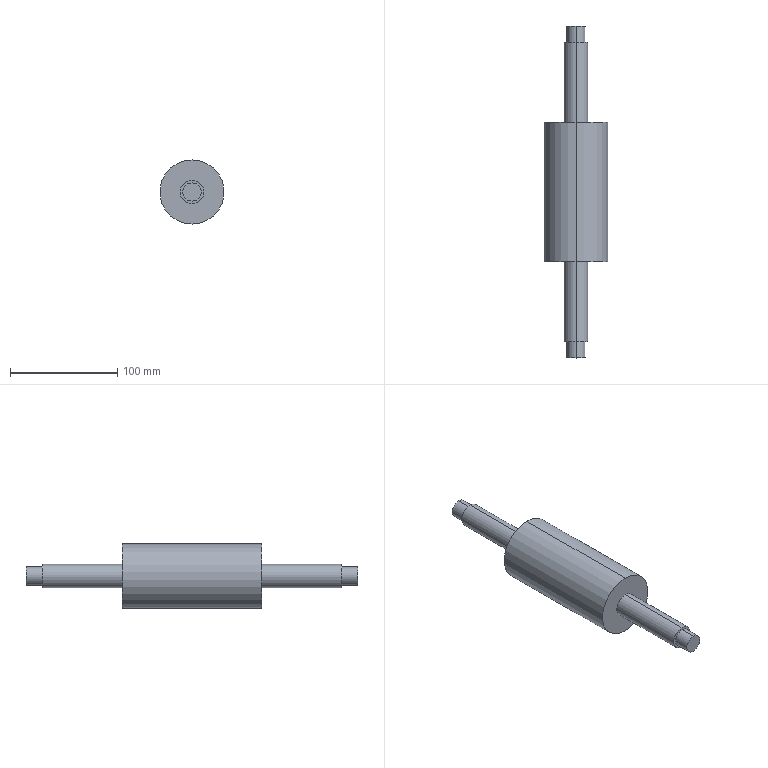Part | STEP file | A14-012 | 1 solid | 16 faces | box 60 x 310 x 60 mm | volume 431396 mm3 | cylinder 10 | plane 6 | commonest cylinder face diameters 17 x4 22 x4 60 x2
STEP:
#1=CARTESIAN_POINT('',(0.,0.,0.));
#2=DIRECTION('',(0.,0.,1.));
#3=DIRECTION('',(1.,0.,0.));
#4=AXIS2_PLACEMENT_3D('',#1,#2,#3);
#5=CARTESIAN_POINT('',(0.,15.,-8.5));
#6=VERTEX_POINT('',#5);
#7=CARTESIAN_POINT('',(0.,15.,8.5));
#8=VERTEX_POINT('',#7);
#9=CARTESIAN_POINT('',(0.,15.,0.));
#10=DIRECTION('',(0.,-1.,0.));
#11=DIRECTION('',(0.,0.,-1.));
#12=AXIS2_PLACEMENT_3D('',#9,#10,#11);
#13=CIRCLE('',#12,8.5);
#14=CARTESIAN_POINT('',(0.,0.,0.));
#15=DIRECTION('',(0.,-1.,0.));
#16=DIRECTION('',(0.,0.,-1.));
#17=AXIS2_PLACEMENT_3D('',#14,#15,#16);
#18=CYLINDRICAL_SURFACE('',#17,8.5);
#19=CARTESIAN_POINT('',(0.,-15.));
#20=DIRECTION('',(1.,0.));
#21=VECTOR('',#20,1.);
#22=LINE('',#19,#21);
#23=(GEOMETRIC_REPRESENTATION_CONTEXT(2)PARAMETRIC_REPRESENTATION_CONTEXT()REPRESENTATION_CONTEXT('',''));
#24=DEFINITIONAL_REPRESENTATION('',(#22),#23);
#25=PCURVE('',#18,#24);
#26=CARTESIAN_POINT('',(11.,15.,0.));
#27=DIRECTION('',(0.,-1.,0.));
#28=DIRECTION('',(0.,0.,-1.));
#29=AXIS2_PLACEMENT_3D('',#26,#27,#28);
#30=PLANE('',#29);
#31=CARTESIAN_POINT('',(0.,-11.));
#32=DIRECTION('',(1.,0.));
#33=AXIS2_PLACEMENT_2D('',#31,#32);
#34=CIRCLE('',#33,8.5);
#35=(GEOMETRIC_REPRESENTATION_CONTEXT(2)PARAMETRIC_REPRESENTATION_CONTEXT()REPRESENTATION_CONTEXT('',''));
#36=DEFINITIONAL_REPRESENTATION('',(#34),#35);
#37=PCURVE('',#30,#36);
#38=SURFACE_CURVE('',#13,(#25,#37),.PCURVE_S1.);
#39=EDGE_CURVE('',#6,#8,#38,.T.);
#40=ORIENTED_EDGE('',*,*,#39,.T.);
#41=CARTESIAN_POINT('',(0.,0.,8.5));
#42=VERTEX_POINT('',#41);
#43=CARTESIAN_POINT('',(0.,0.,8.5));
#44=DIRECTION('',(0.,-1.,0.));
#45=VECTOR('',#44,1.);
#46=LINE('',#43,#45);
#47=CARTESIAN_POINT('',(3.142,0.));
#48=DIRECTION('',(0.,1.));
#49=VECTOR('',#48,1.);
#50=LINE('',#47,#49);
#51=(GEOMETRIC_REPRESENTATION_CONTEXT(2)PARAMETRIC_REPRESENTATION_CONTEXT()REPRESENTATION_CONTEXT('',''));
#52=DEFINITIONAL_REPRESENTATION('',(#50),#51);
#53=PCURVE('',#18,#52);
#54=CARTESIAN_POINT('',(0.,0.,0.));
#55=DIRECTION('',(0.,-1.,0.));
#56=DIRECTION('',(0.,0.,-1.));
#57=AXIS2_PLACEMENT_3D('',#54,#55,#56);
#58=CYLINDRICAL_SURFACE('',#57,8.5);
#59=CARTESIAN_POINT('',(3.142,0.));
#60=DIRECTION('',(0.,1.));
#61=VECTOR('',#60,1.);
#62=LINE('',#59,#61);
#63=(GEOMETRIC_REPRESENTATION_CONTEXT(2)PARAMETRIC_REPRESENTATION_CONTEXT()REPRESENTATION_CONTEXT('',''));
#64=DEFINITIONAL_REPRESENTATION('',(#62),#63);
#65=PCURVE('',#58,#64);
#66=SURFACE_CURVE('',#46,(#53,#65),.PCURVE_S1.);
#67=EDGE_CURVE('',#8,#42,#66,.T.);
#68=ORIENTED_EDGE('',*,*,#67,.T.);
#69=CARTESIAN_POINT('',(0.,0.,-8.5));
#70=VERTEX_POINT('',#69);
#71=CARTESIAN_POINT('',(0.,0.,0.));
#72=DIRECTION('',(0.,-1.,0.));
#73=DIRECTION('',(0.,0.,-1.));
#74=AXIS2_PLACEMENT_3D('',#71,#72,#73);
#75=CIRCLE('',#74,8.5);
#76=CARTESIAN_POINT('',(0.,0.));
#77=DIRECTION('',(1.,0.));
#78=VECTOR('',#77,1.);
#79=LINE('',#76,#78);
#80=(GEOMETRIC_REPRESENTATION_CONTEXT(2)PARAMETRIC_REPRESENTATION_CONTEXT()REPRESENTATION_CONTEXT('',''));
#81=DEFINITIONAL_REPRESENTATION('',(#79),#80);
#82=PCURVE('',#18,#81);
#83=CARTESIAN_POINT('',(8.5,0.,0.));
#84=DIRECTION('',(0.,-1.,0.));
#85=DIRECTION('',(0.,0.,-1.));
#86=AXIS2_PLACEMENT_3D('',#83,#84,#85);
#87=PLANE('',#86);
#88=CARTESIAN_POINT('',(0.,-8.5));
#89=DIRECTION('',(1.,0.));
#90=AXIS2_PLACEMENT_2D('',#88,#89);
#91=CIRCLE('',#90,8.5);
#92=(GEOMETRIC_REPRESENTATION_CONTEXT(2)PARAMETRIC_REPRESENTATION_CONTEXT()REPRESENTATION_CONTEXT('',''));
#93=DEFINITIONAL_REPRESENTATION('',(#91),#92);
#94=PCURVE('',#87,#93);
#95=SURFACE_CURVE('',#75,(#82,#94),.PCURVE_S1.);
#96=EDGE_CURVE('',#70,#42,#95,.T.);
#97=ORIENTED_EDGE('',*,*,#96,.F.);
#98=CARTESIAN_POINT('',(0.,0.,-8.5));
#99=DIRECTION('',(0.,-1.,0.));
#100=VECTOR('',#99,1.);
#101=LINE('',#98,#100);
#102=CARTESIAN_POINT('',(0.,0.));
#103=DIRECTION('',(0.,1.));
#104=VECTOR('',#103,1.);
#105=LINE('',#102,#104);
#106=(GEOMETRIC_REPRESENTATION_CONTEXT(2)PARAMETRIC_REPRESENTATION_CONTEXT()REPRESENTATION_CONTEXT('',''));
#107=DEFINITIONAL_REPRESENTATION('',(#105),#106);
#108=PCURVE('',#18,#107);
#109=CARTESIAN_POINT('',(6.283,0.));
#110=DIRECTION('',(0.,1.));
#111=VECTOR('',#110,1.);
#112=LINE('',#109,#111);
#113=(GEOMETRIC_REPRESENTATION_CONTEXT(2)PARAMETRIC_REPRESENTATION_CONTEXT()REPRESENTATION_CONTEXT('',''));
#114=DEFINITIONAL_REPRESENTATION('',(#112),#113);
#115=PCURVE('',#58,#114);
#116=SURFACE_CURVE('',#101,(#108,#115),.PCURVE_S1.);
#117=EDGE_CURVE('',#6,#70,#116,.T.);
#118=ORIENTED_EDGE('',*,*,#117,.F.);
#119=EDGE_LOOP('',(#40,#68,#97,#118));
#120=FACE_BOUND('',#119,.T.);
#121=ADVANCED_FACE('',(#120),#18,.T.);
#122=CARTESIAN_POINT('',(0.,90.,-11.));
#123=VERTEX_POINT('',#122);
#124=CARTESIAN_POINT('',(0.,90.,11.));
#125=VERTEX_POINT('',#124);
#126=CARTESIAN_POINT('',(0.,90.,0.));
#127=DIRECTION('',(0.,-1.,0.));
#128=DIRECTION('',(0.,0.,-1.));
#129=AXIS2_PLACEMENT_3D('',#126,#127,#128);
#130=CIRCLE('',#129,11.);
#131=CARTESIAN_POINT('',(0.,0.,0.));
#132=DIRECTION('',(0.,-1.,0.));
#133=DIRECTION('',(0.,0.,-1.));
#134=AXIS2_PLACEMENT_3D('',#131,#132,#133);
#135=CYLINDRICAL_SURFACE('',#134,11.);
#136=CARTESIAN_POINT('',(0.,-90.));
#137=DIRECTION('',(1.,0.));
#138=VECTOR('',#137,1.);
#139=LINE('',#136,#138);
#140=(GEOMETRIC_REPRESENTATION_CONTEXT(2)PARAMETRIC_REPRESENTATION_CONTEXT()REPRESENTATION_CONTEXT('',''));
#141=DEFINITIONAL_REPRESENTATION('',(#139),#140);
#142=PCURVE('',#135,#141);
#143=CARTESIAN_POINT('',(30.,90.,0.));
#144=DIRECTION('',(0.,-1.,0.));
#145=DIRECTION('',(0.,0.,-1.));
#146=AXIS2_PLACEMENT_3D('',#143,#144,#145);
#147=PLANE('',#146);
#148=CARTESIAN_POINT('',(0.,-30.));
#149=DIRECTION('',(1.,0.));
#150=AXIS2_PLACEMENT_2D('',#148,#149);
#151=CIRCLE('',#150,11.);
#152=(GEOMETRIC_REPRESENTATION_CONTEXT(2)PARAMETRIC_REPRESENTATION_CONTEXT()REPRESENTATION_CONTEXT('',''));
#153=DEFINITIONAL_REPRESENTATION('',(#151),#152);
#154=PCURVE('',#147,#153);
#155=SURFACE_CURVE('',#130,(#142,#154),.PCURVE_S1.);
#156=EDGE_CURVE('',#123,#125,#155,.T.);
#157=ORIENTED_EDGE('',*,*,#156,.T.);
#158=CARTESIAN_POINT('',(0.,15.,11.));
#159=VERTEX_POINT('',#158);
#160=CARTESIAN_POINT('',(0.,0.,11.));
#161=DIRECTION('',(0.,-1.,0.));
#162=VECTOR('',#161,1.);
#163=LINE('',#160,#162);
#164=CARTESIAN_POINT('',(3.142,0.));
#165=DIRECTION('',(0.,1.));
#166=VECTOR('',#165,1.);
#167=LINE('',#164,#166);
#168=(GEOMETRIC_REPRESENTATION_CONTEXT(2)PARAMETRIC_REPRESENTATION_CONTEXT()REPRESENTATION_CONTEXT('',''));
#169=DEFINITIONAL_REPRESENTATION('',(#167),#168);
#170=PCURVE('',#135,#169);
#171=CARTESIAN_POINT('',(0.,0.,0.));
#172=DIRECTION('',(0.,-1.,0.));
#173=DIRECTION('',(0.,0.,-1.));
#174=AXIS2_PLACEMENT_3D('',#171,#172,#173);
#175=CYLINDRICAL_SURFACE('',#174,11.);
#176=CARTESIAN_POINT('',(3.142,0.));
#177=DIRECTION('',(0.,1.));
#178=VECTOR('',#177,1.);
#179=LINE('',#176,#178);
#180=(GEOMETRIC_REPRESENTATION_CONTEXT(2)PARAMETRIC_REPRESENTATION_CONTEXT()REPRESENTATION_CONTEXT('',''));
#181=DEFINITIONAL_REPRESENTATION('',(#179),#180);
#182=PCURVE('',#175,#181);
#183=SURFACE_CURVE('',#163,(#170,#182),.PCURVE_S1.);
#184=EDGE_CURVE('',#125,#159,#183,.T.);
#185=ORIENTED_EDGE('',*,*,#184,.T.);
#186=CARTESIAN_POINT('',(0.,15.,-11.));
#187=VERTEX_POINT('',#186);
#188=CARTESIAN_POINT('',(0.,15.,0.));
#189=DIRECTION('',(0.,-1.,0.));
#190=DIRECTION('',(0.,0.,-1.));
#191=AXIS2_PLACEMENT_3D('',#188,#189,#190);
#192=CIRCLE('',#191,11.);
#193=CARTESIAN_POINT('',(0.,-15.));
#194=DIRECTION('',(1.,0.));
#195=VECTOR('',#194,1.);
#196=LINE('',#193,#195);
#197=(GEOMETRIC_REPRESENTATION_CONTEXT(2)PARAMETRIC_REPRESENTATION_CONTEXT()REPRESENTATION_CONTEXT('',''));
#198=DEFINITIONAL_REPRESENTATION('',(#196),#197);
#199=PCURVE('',#135,#198);
#200=CARTESIAN_POINT('',(0.,-11.));
#201=DIRECTION('',(1.,0.));
#202=AXIS2_PLACEMENT_2D('',#200,#201);
#203=CIRCLE('',#202,11.);
#204=(GEOMETRIC_REPRESENTATION_CONTEXT(2)PARAMETRIC_REPRESENTATION_CONTEXT()REPRESENTATION_CONTEXT('',''));
#205=DEFINITIONAL_REPRESENTATION('',(#203),#204);
#206=PCURVE('',#30,#205);
#207=SURFACE_CURVE('',#192,(#199,#206),.PCURVE_S1.);
#208=EDGE_CURVE('',#187,#159,#207,.T.);
#209=ORIENTED_EDGE('',*,*,#208,.F.);
#210=CARTESIAN_POINT('',(0.,0.,-11.));
#211=DIRECTION('',(0.,-1.,0.));
#212=VECTOR('',#211,1.);
#213=LINE('',#210,#212);
#214=CARTESIAN_POINT('',(0.,0.));
#215=DIRECTION('',(0.,1.));
#216=VECTOR('',#215,1.);
#217=LINE('',#214,#216);
#218=(GEOMETRIC_REPRESENTATION_CONTEXT(2)PARAMETRIC_REPRESENTATION_CONTEXT()REPRESENTATION_CONTEXT('',''));
#219=DEFINITIONAL_REPRESENTATION('',(#217),#218);
#220=PCURVE('',#135,#219);
#221=CARTESIAN_POINT('',(6.283,0.));
#222=DIRECTION('',(0.,1.));
#223=VECTOR('',#222,1.);
#224=LINE('',#221,#223);
#225=(GEOMETRIC_REPRESENTATION_CONTEXT(2)PARAMETRIC_REPRESENTATION_CONTEXT()REPRESENTATION_CONTEXT('',''));
#226=DEFINITIONAL_REPRESENTATION('',(#224),#225);
#227=PCURVE('',#175,#226);
#228=SURFACE_CURVE('',#213,(#220,#227),.PCURVE_S1.);
#229=EDGE_CURVE('',#123,#187,#228,.T.);
#230=ORIENTED_EDGE('',*,*,#229,.F.);
#231=EDGE_LOOP('',(#157,#185,#209,#230));
#232=FACE_BOUND('',#231,.T.);
#233=ADVANCED_FACE('',(#232),#135,.T.);
#234=CARTESIAN_POINT('',(0.,220.,-30.));
#235=VERTEX_POINT('',#234);
#236=CARTESIAN_POINT('',(0.,220.,30.));
#237=VERTEX_POINT('',#236);
#238=CARTESIAN_POINT('',(0.,220.,0.));
#239=DIRECTION('',(0.,-1.,0.));
#240=DIRECTION('',(0.,0.,-1.));
#241=AXIS2_PLACEMENT_3D('',#238,#239,#240);
#242=CIRCLE('',#241,30.);
#243=CARTESIAN_POINT('',(0.,0.,0.));
#244=DIRECTION('',(0.,-1.,0.));
#245=DIRECTION('',(0.,0.,-1.));
#246=AXIS2_PLACEMENT_3D('',#243,#244,#245);
#247=CYLINDRICAL_SURFACE('',#246,30.);
#248=CARTESIAN_POINT('',(0.,-220.));
#249=DIRECTION('',(1.,0.));
#250=VECTOR('',#249,1.);
#251=LINE('',#248,#250);
#252=(GEOMETRIC_REPRESENTATION_CONTEXT(2)PARAMETRIC_REPRESENTATION_CONTEXT()REPRESENTATION_CONTEXT('',''));
#253=DEFINITIONAL_REPRESENTATION('',(#251),#252);
#254=PCURVE('',#247,#253);
#255=CARTESIAN_POINT('',(11.,220.,0.));
#256=DIRECTION('',(0.,1.,0.));
#257=DIRECTION('',(0.,0.,1.));
#258=AXIS2_PLACEMENT_3D('',#255,#256,#257);
#259=PLANE('',#258);
#260=CARTESIAN_POINT('',(-30.,-11.));
#261=CARTESIAN_POINT('',(-30.,40.962));
#262=CARTESIAN_POINT('',(15.,14.981));
#263=CARTESIAN_POINT('',(60.,-11.));
#264=CARTESIAN_POINT('',(15.,-36.981));
#265=CARTESIAN_POINT('',(-30.,-62.962));
#266=CARTESIAN_POINT('',(-30.,-11.));
#267=(BOUNDED_CURVE()B_SPLINE_CURVE(2,(#260,#261,#262,#263,#264,#265,#266),.UNSPECIFIED.,.T.,.F.)B_SPLINE_CURVE_WITH_KNOTS((1,2,2,2,2,1),(-2.094,0.,2.094,4.189,6.283,8.378),.UNSPECIFIED.)CURVE()GEOMETRIC_REPRESENTATION_ITEM()RATIONAL_B_SPLINE_CURVE((1.,0.5,1.,0.5,1.,0.5,1.))REPRESENTATION_ITEM(''));
#268=(GEOMETRIC_REPRESENTATION_CONTEXT(2)PARAMETRIC_REPRESENTATION_CONTEXT()REPRESENTATION_CONTEXT('',''));
#269=DEFINITIONAL_REPRESENTATION('',(#267),#268);
#270=PCURVE('',#259,#269);
#271=SURFACE_CURVE('',#242,(#254,#270),.PCURVE_S1.);
#272=EDGE_CURVE('',#235,#237,#271,.T.);
#273=ORIENTED_EDGE('',*,*,#272,.T.);
#274=CARTESIAN_POINT('',(0.,90.,30.));
#275=VERTEX_POINT('',#274);
#276=CARTESIAN_POINT('',(0.,0.,30.));
#277=DIRECTION('',(0.,-1.,0.));
#278=VECTOR('',#277,1.);
#279=LINE('',#276,#278);
#280=CARTESIAN_POINT('',(3.142,0.));
#281=DIRECTION('',(0.,1.));
#282=VECTOR('',#281,1.);
#283=LINE('',#280,#282);
#284=(GEOMETRIC_REPRESENTATION_CONTEXT(2)PARAMETRIC_REPRESENTATION_CONTEXT()REPRESENTATION_CONTEXT('',''));
#285=DEFINITIONAL_REPRESENTATION('',(#283),#284);
#286=PCURVE('',#247,#285);
#287=CARTESIAN_POINT('',(0.,0.,0.));
#288=DIRECTION('',(0.,-1.,0.));
#289=DIRECTION('',(0.,0.,-1.));
#290=AXIS2_PLACEMENT_3D('',#287,#288,#289);
#291=CYLINDRICAL_SURFACE('',#290,30.);
#292=CARTESIAN_POINT('',(3.142,0.));
#293=DIRECTION('',(0.,1.));
#294=VECTOR('',#293,1.);
#295=LINE('',#292,#294);
#296=(GEOMETRIC_REPRESENTATION_CONTEXT(2)PARAMETRIC_REPRESENTATION_CONTEXT()REPRESENTATION_CONTEXT('',''));
#297=DEFINITIONAL_REPRESENTATION('',(#295),#296);
#298=PCURVE('',#291,#297);
#299=SURFACE_CURVE('',#279,(#286,#298),.PCURVE_S1.);
#300=EDGE_CURVE('',#237,#275,#299,.T.);
#301=ORIENTED_EDGE('',*,*,#300,.T.);
#302=CARTESIAN_POINT('',(0.,90.,-30.));
#303=VERTEX_POINT('',#302);
#304=CARTESIAN_POINT('',(0.,90.,0.));
#305=DIRECTION('',(0.,-1.,0.));
#306=DIRECTION('',(0.,0.,-1.));
#307=AXIS2_PLACEMENT_3D('',#304,#305,#306);
#308=CIRCLE('',#307,30.);
#309=CARTESIAN_POINT('',(0.,-90.));
#310=DIRECTION('',(1.,0.));
#311=VECTOR('',#310,1.);
#312=LINE('',#309,#311);
#313=(GEOMETRIC_REPRESENTATION_CONTEXT(2)PARAMETRIC_REPRESENTATION_CONTEXT()REPRESENTATION_CONTEXT('',''));
#314=DEFINITIONAL_REPRESENTATION('',(#312),#313);
#315=PCURVE('',#247,#314);
#316=CARTESIAN_POINT('',(0.,-30.));
#317=DIRECTION('',(1.,0.));
#318=AXIS2_PLACEMENT_2D('',#316,#317);
#319=CIRCLE('',#318,30.);
#320=(GEOMETRIC_REPRESENTATION_CONTEXT(2)PARAMETRIC_REPRESENTATION_CONTEXT()REPRESENTATION_CONTEXT('',''));
#321=DEFINITIONAL_REPRESENTATION('',(#319),#320);
#322=PCURVE('',#147,#321);
#323=SURFACE_CURVE('',#308,(#315,#322),.PCURVE_S1.);
#324=EDGE_CURVE('',#303,#275,#323,.T.);
#325=ORIENTED_EDGE('',*,*,#324,.F.);
#326=CARTESIAN_POINT('',(0.,0.,-30.));
#327=DIRECTION('',(0.,-1.,0.));
#328=VECTOR('',#327,1.);
#329=LINE('',#326,#328);
#330=CARTESIAN_POINT('',(0.,0.));
#331=DIRECTION('',(0.,1.));
#332=VECTOR('',#331,1.);
#333=LINE('',#330,#332);
#334=(GEOMETRIC_REPRESENTATION_CONTEXT(2)PARAMETRIC_REPRESENTATION_CONTEXT()REPRESENTATION_CONTEXT('',''));
#335=DEFINITIONAL_REPRESENTATION('',(#333),#334);
#336=PCURVE('',#247,#335);
#337=CARTESIAN_POINT('',(6.283,0.));
#338=DIRECTION('',(0.,1.));
#339=VECTOR('',#338,1.);
#340=LINE('',#337,#339);
#341=(GEOMETRIC_REPRESENTATION_CONTEXT(2)PARAMETRIC_REPRESENTATION_CONTEXT()REPRESENTATION_CONTEXT('',''));
#342=DEFINITIONAL_REPRESENTATION('',(#340),#341);
#343=PCURVE('',#291,#342);
#344=SURFACE_CURVE('',#329,(#336,#343),.PCURVE_S1.);
#345=EDGE_CURVE('',#235,#303,#344,.T.);
#346=ORIENTED_EDGE('',*,*,#345,.F.);
#347=EDGE_LOOP('',(#273,#301,#325,#346));
#348=FACE_BOUND('',#347,.T.);
#349=ADVANCED_FACE('',(#348),#247,.T.);
#350=CARTESIAN_POINT('',(0.,295.,-11.));
#351=VERTEX_POINT('',#350);
#352=CARTESIAN_POINT('',(0.,295.,11.));
#353=VERTEX_POINT('',#352);
#354=CARTESIAN_POINT('',(0.,295.,0.));
#355=DIRECTION('',(0.,-1.,0.));
#356=DIRECTION('',(0.,0.,-1.));
#357=AXIS2_PLACEMENT_3D('',#354,#355,#356);
#358=CIRCLE('',#357,11.);
#359=CARTESIAN_POINT('',(0.,0.,0.));
#360=DIRECTION('',(0.,-1.,0.));
#361=DIRECTION('',(0.,0.,-1.));
#362=AXIS2_PLACEMENT_3D('',#359,#360,#361);
#363=CYLINDRICAL_SURFACE('',#362,11.);
#364=CARTESIAN_POINT('',(0.,-295.));
#365=DIRECTION('',(1.,0.));
#366=VECTOR('',#365,1.);
#367=LINE('',#364,#366);
#368=(GEOMETRIC_REPRESENTATION_CONTEXT(2)PARAMETRIC_REPRESENTATION_CONTEXT()REPRESENTATION_CONTEXT('',''));
#369=DEFINITIONAL_REPRESENTATION('',(#367),#368);
#370=PCURVE('',#363,#369);
#371=CARTESIAN_POINT('',(8.5,295.,0.));
#372=DIRECTION('',(0.,1.,0.));
#373=DIRECTION('',(0.,0.,1.));
#374=AXIS2_PLACEMENT_3D('',#371,#372,#373);
#375=PLANE('',#374);
#376=CARTESIAN_POINT('',(-11.,-8.5));
#377=CARTESIAN_POINT('',(-11.,10.553));
#378=CARTESIAN_POINT('',(5.5,1.026));
#379=CARTESIAN_POINT('',(22.,-8.5));
#380=CARTESIAN_POINT('',(5.5,-18.026));
#381=CARTESIAN_POINT('',(-11.,-27.553));
#382=CARTESIAN_POINT('',(-11.,-8.5));
#383=(BOUNDED_CURVE()B_SPLINE_CURVE(2,(#376,#377,#378,#379,#380,#381,#382),.UNSPECIFIED.,.T.,.F.)B_SPLINE_CURVE_WITH_KNOTS((1,2,2,2,2,1),(-2.094,0.,2.094,4.189,6.283,8.378),.UNSPECIFIED.)CURVE()GEOMETRIC_REPRESENTATION_ITEM()RATIONAL_B_SPLINE_CURVE((1.,0.5,1.,0.5,1.,0.5,1.))REPRESENTATION_ITEM(''));
#384=(GEOMETRIC_REPRESENTATION_CONTEXT(2)PARAMETRIC_REPRESENTATION_CONTEXT()REPRESENTATION_CONTEXT('',''));
#385=DEFINITIONAL_REPRESENTATION('',(#383),#384);
#386=PCURVE('',#375,#385);
#387=SURFACE_CURVE('',#358,(#370,#386),.PCURVE_S1.);
#388=EDGE_CURVE('',#351,#353,#387,.T.);
#389=ORIENTED_EDGE('',*,*,#388,.T.);
#390=CARTESIAN_POINT('',(0.,220.,11.));
#391=VERTEX_POINT('',#390);
#392=CARTESIAN_POINT('',(0.,0.,11.));
#393=DIRECTION('',(0.,-1.,0.));
#394=VECTOR('',#393,1.);
#395=LINE('',#392,#394);
#396=CARTESIAN_POINT('',(3.142,0.));
#397=DIRECTION('',(0.,1.));
#398=VECTOR('',#397,1.);
#399=LINE('',#396,#398);
#400=(GEOMETRIC_REPRESENTATION_CONTEXT(2)PARAMETRIC_REPRESENTATION_CONTEXT()REPRESENTATION_CONTEXT('',''));
#401=DEFINITIONAL_REPRESENTATION('',(#399),#400);
#402=PCURVE('',#363,#401);
#403=CARTESIAN_POINT('',(0.,0.,0.));
#404=DIRECTION('',(0.,-1.,0.));
#405=DIRECTION('',(0.,0.,-1.));
#406=AXIS2_PLACEMENT_3D('',#403,#404,#405);
#407=CYLINDRICAL_SURFACE('',#406,11.);
#408=CARTESIAN_POINT('',(3.142,0.));
#409=DIRECTION('',(0.,1.));
#410=VECTOR('',#409,1.);
#411=LINE('',#408,#410);
#412=(GEOMETRIC_REPRESENTATION_CONTEXT(2)PARAMETRIC_REPRESENTATION_CONTEXT()REPRESENTATION_CONTEXT('',''));
#413=DEFINITIONAL_REPRESENTATION('',(#411),#412);
#414=PCURVE('',#407,#413);
#415=SURFACE_CURVE('',#395,(#402,#414),.PCURVE_S1.);
#416=EDGE_CURVE('',#353,#391,#415,.T.);
#417=ORIENTED_EDGE('',*,*,#416,.T.);
#418=CARTESIAN_POINT('',(0.,220.,-11.));
#419=VERTEX_POINT('',#418);
#420=CARTESIAN_POINT('',(0.,220.,0.));
#421=DIRECTION('',(0.,-1.,0.));
#422=DIRECTION('',(0.,0.,-1.));
#423=AXIS2_PLACEMENT_3D('',#420,#421,#422);
#424=CIRCLE('',#423,11.);
#425=CARTESIAN_POINT('',(0.,-220.));
#426=DIRECTION('',(1.,0.));
#427=VECTOR('',#426,1.);
#428=LINE('',#425,#427);
#429=(GEOMETRIC_REPRESENTATION_CONTEXT(2)PARAMETRIC_REPRESENTATION_CONTEXT()REPRESENTATION_CONTEXT('',''));
#430=DEFINITIONAL_REPRESENTATION('',(#428),#429);
#431=PCURVE('',#363,#430);
#432=CARTESIAN_POINT('',(-11.,-11.));
#433=CARTESIAN_POINT('',(-11.,8.053));
#434=CARTESIAN_POINT('',(5.5,-1.474));
#435=CARTESIAN_POINT('',(22.,-11.));
#436=CARTESIAN_POINT('',(5.5,-20.526));
#437=CARTESIAN_POINT('',(-11.,-30.053));
#438=CARTESIAN_POINT('',(-11.,-11.));
#439=(BOUNDED_CURVE()B_SPLINE_CURVE(2,(#432,#433,#434,#435,#436,#437,#438),.UNSPECIFIED.,.T.,.F.)B_SPLINE_CURVE_WITH_KNOTS((1,2,2,2,2,1),(-2.094,0.,2.094,4.189,6.283,8.378),.UNSPECIFIED.)CURVE()GEOMETRIC_REPRESENTATION_ITEM()RATIONAL_B_SPLINE_CURVE((1.,0.5,1.,0.5,1.,0.5,1.))REPRESENTATION_ITEM(''));
#440=(GEOMETRIC_REPRESENTATION_CONTEXT(2)PARAMETRIC_REPRESENTATION_CONTEXT()REPRESENTATION_CONTEXT('',''));
#441=DEFINITIONAL_REPRESENTATION('',(#439),#440);
#442=PCURVE('',#259,#441);
#443=SURFACE_CURVE('',#424,(#431,#442),.PCURVE_S1.);
#444=EDGE_CURVE('',#419,#391,#443,.T.);
#445=ORIENTED_EDGE('',*,*,#444,.F.);
#446=CARTESIAN_POINT('',(0.,0.,-11.));
#447=DIRECTION('',(0.,-1.,0.));
#448=VECTOR('',#447,1.);
#449=LINE('',#446,#448);
#450=CARTESIAN_POINT('',(0.,0.));
#451=DIRECTION('',(0.,1.));
#452=VECTOR('',#451,1.);
#453=LINE('',#450,#452);
#454=(GEOMETRIC_REPRESENTATION_CONTEXT(2)PARAMETRIC_REPRESENTATION_CONTEXT()REPRESENTATION_CONTEXT('',''));
#455=DEFINITIONAL_REPRESENTATION('',(#453),#454);
#456=PCURVE('',#363,#455);
#457=CARTESIAN_POINT('',(6.283,0.));
#458=DIRECTION('',(0.,1.));
#459=VECTOR('',#458,1.);
#460=LINE('',#457,#459);
#461=(GEOMETRIC_REPRESENTATION_CONTEXT(2)PARAMETRIC_REPRESENTATION_CONTEXT()REPRESENTATION_CONTEXT('',''));
#462=DEFINITIONAL_REPRESENTATION('',(#460),#461);
#463=PCURVE('',#407,#462);
#464=SURFACE_CURVE('',#449,(#456,#463),.PCURVE_S1.);
#465=EDGE_CURVE('',#351,#419,#464,.T.);
#466=ORIENTED_EDGE('',*,*,#465,.F.);
#467=EDGE_LOOP('',(#389,#417,#445,#466));
#468=FACE_BOUND('',#467,.T.);
#469=ADVANCED_FACE('',(#468),#363,.T.);
#470=CARTESIAN_POINT('',(0.,310.,-8.5));
#471=VERTEX_POINT('',#470);
#472=CARTESIAN_POINT('',(0.,310.,8.5));
#473=VERTEX_POINT('',#472);
#474=CARTESIAN_POINT('',(0.,310.,0.));
#475=DIRECTION('',(0.,-1.,0.));
#476=DIRECTION('',(0.,0.,-1.));
#477=AXIS2_PLACEMENT_3D('',#474,#475,#476);
#478=CIRCLE('',#477,8.5);
#479=CARTESIAN_POINT('',(0.,0.,0.));
#480=DIRECTION('',(0.,-1.,0.));
#481=DIRECTION('',(0.,0.,-1.));
#482=AXIS2_PLACEMENT_3D('',#479,#480,#481);
#483=CYLINDRICAL_SURFACE('',#482,8.5);
#484=CARTESIAN_POINT('',(0.,-310.));
#485=DIRECTION('',(1.,0.));
#486=VECTOR('',#485,1.);
#487=LINE('',#484,#486);
#488=(GEOMETRIC_REPRESENTATION_CONTEXT(2)PARAMETRIC_REPRESENTATION_CONTEXT()REPRESENTATION_CONTEXT('',''));
#489=DEFINITIONAL_REPRESENTATION('',(#487),#488);
#490=PCURVE('',#483,#489);
#491=CARTESIAN_POINT('',(0.,310.,0.));
#492=DIRECTION('',(0.,1.,0.));
#493=DIRECTION('',(0.,0.,1.));
#494=AXIS2_PLACEMENT_3D('',#491,#492,#493);
#495=PLANE('',#494);
#496=CARTESIAN_POINT('',(-8.5,0.));
#497=CARTESIAN_POINT('',(-8.5,14.722));
#498=CARTESIAN_POINT('',(4.25,7.361));
#499=CARTESIAN_POINT('',(17.,0.));
#500=CARTESIAN_POINT('',(4.25,-7.361));
#501=CARTESIAN_POINT('',(-8.5,-14.722));
#502=CARTESIAN_POINT('',(-8.5,0.));
#503=(BOUNDED_CURVE()B_SPLINE_CURVE(2,(#496,#497,#498,#499,#500,#501,#502),.UNSPECIFIED.,.T.,.F.)B_SPLINE_CURVE_WITH_KNOTS((1,2,2,2,2,1),(-2.094,0.,2.094,4.189,6.283,8.378),.UNSPECIFIED.)CURVE()GEOMETRIC_REPRESENTATION_ITEM()RATIONAL_B_SPLINE_CURVE((1.,0.5,1.,0.5,1.,0.5,1.))REPRESENTATION_ITEM(''));
#504=(GEOMETRIC_REPRESENTATION_CONTEXT(2)PARAMETRIC_REPRESENTATION_CONTEXT()REPRESENTATION_CONTEXT('',''));
#505=DEFINITIONAL_REPRESENTATION('',(#503),#504);
#506=PCURVE('',#495,#505);
#507=SURFACE_CURVE('',#478,(#490,#506),.PCURVE_S1.);
#508=EDGE_CURVE('',#471,#473,#507,.T.);
#509=ORIENTED_EDGE('',*,*,#508,.T.);
#510=CARTESIAN_POINT('',(0.,295.,8.5));
#511=VERTEX_POINT('',#510);
#512=CARTESIAN_POINT('',(0.,0.,8.5));
#513=DIRECTION('',(0.,-1.,0.));
#514=VECTOR('',#513,1.);
#515=LINE('',#512,#514);
#516=CARTESIAN_POINT('',(3.142,0.));
#517=DIRECTION('',(0.,1.));
#518=VECTOR('',#517,1.);
#519=LINE('',#516,#518);
#520=(GEOMETRIC_REPRESENTATION_CONTEXT(2)PARAMETRIC_REPRESENTATION_CONTEXT()REPRESENTATION_CONTEXT('',''));
#521=DEFINITIONAL_REPRESENTATION('',(#519),#520);
#522=PCURVE('',#483,#521);
#523=CARTESIAN_POINT('',(0.,0.,0.));
#524=DIRECTION('',(0.,-1.,0.));
#525=DIRECTION('',(0.,0.,-1.));
#526=AXIS2_PLACEMENT_3D('',#523,#524,#525);
#527=CYLINDRICAL_SURFACE('',#526,8.5);
#528=CARTESIAN_POINT('',(3.142,0.));
#529=DIRECTION('',(0.,1.));
#530=VECTOR('',#529,1.);
#531=LINE('',#528,#530);
#532=(GEOMETRIC_REPRESENTATION_CONTEXT(2)PARAMETRIC_REPRESENTATION_CONTEXT()REPRESENTATION_CONTEXT('',''));
#533=DEFINITIONAL_REPRESENTATION('',(#531),#532);
#534=PCURVE('',#527,#533);
#535=SURFACE_CURVE('',#515,(#522,#534),.PCURVE_S1.);
#536=EDGE_CURVE('',#473,#511,#535,.T.);
#537=ORIENTED_EDGE('',*,*,#536,.T.);
#538=CARTESIAN_POINT('',(0.,295.,-8.5));
#539=VERTEX_POINT('',#538);
#540=CARTESIAN_POINT('',(0.,295.,0.));
#541=DIRECTION('',(0.,-1.,0.));
#542=DIRECTION('',(0.,0.,-1.));
#543=AXIS2_PLACEMENT_3D('',#540,#541,#542);
#544=CIRCLE('',#543,8.5);
#545=CARTESIAN_POINT('',(0.,-295.));
#546=DIRECTION('',(1.,0.));
#547=VECTOR('',#546,1.);
#548=LINE('',#545,#547);
#549=(GEOMETRIC_REPRESENTATION_CONTEXT(2)PARAMETRIC_REPRESENTATION_CONTEXT()REPRESENTATION_CONTEXT('',''));
#550=DEFINITIONAL_REPRESENTATION('',(#548),#549);
#551=PCURVE('',#483,#550);
#552=CARTESIAN_POINT('',(-8.5,-8.5));
#553=CARTESIAN_POINT('',(-8.5,6.222));
#554=CARTESIAN_POINT('',(4.25,-1.139));
#555=CARTESIAN_POINT('',(17.,-8.5));
#556=CARTESIAN_POINT('',(4.25,-15.861));
#557=CARTESIAN_POINT('',(-8.5,-23.222));
#558=CARTESIAN_POINT('',(-8.5,-8.5));
#559=(BOUNDED_CURVE()B_SPLINE_CURVE(2,(#552,#553,#554,#555,#556,#557,#558),.UNSPECIFIED.,.T.,.F.)B_SPLINE_CURVE_WITH_KNOTS((1,2,2,2,2,1),(-2.094,0.,2.094,4.189,6.283,8.378),.UNSPECIFIED.)CURVE()GEOMETRIC_REPRESENTATION_ITEM()RATIONAL_B_SPLINE_CURVE((1.,0.5,1.,0.5,1.,0.5,1.))REPRESENTATION_ITEM(''));
#560=(GEOMETRIC_REPRESENTATION_CONTEXT(2)PARAMETRIC_REPRESENTATION_CONTEXT()REPRESENTATION_CONTEXT('',''));
#561=DEFINITIONAL_REPRESENTATION('',(#559),#560);
#562=PCURVE('',#375,#561);
#563=SURFACE_CURVE('',#544,(#551,#562),.PCURVE_S1.);
#564=EDGE_CURVE('',#539,#511,#563,.T.);
#565=ORIENTED_EDGE('',*,*,#564,.F.);
#566=CARTESIAN_POINT('',(0.,0.,-8.5));
#567=DIRECTION('',(0.,-1.,0.));
#568=VECTOR('',#567,1.);
#569=LINE('',#566,#568);
#570=CARTESIAN_POINT('',(0.,0.));
#571=DIRECTION('',(0.,1.));
#572=VECTOR('',#571,1.);
#573=LINE('',#570,#572);
#574=(GEOMETRIC_REPRESENTATION_CONTEXT(2)PARAMETRIC_REPRESENTATION_CONTEXT()REPRESENTATION_CONTEXT('',''));
#575=DEFINITIONAL_REPRESENTATION('',(#573),#574);
#576=PCURVE('',#483,#575);
#577=CARTESIAN_POINT('',(6.283,0.));
#578=DIRECTION('',(0.,1.));
#579=VECTOR('',#578,1.);
#580=LINE('',#577,#579);
#581=(GEOMETRIC_REPRESENTATION_CONTEXT(2)PARAMETRIC_REPRESENTATION_CONTEXT()REPRESENTATION_CONTEXT('',''));
#582=DEFINITIONAL_REPRESENTATION('',(#580),#581);
#583=PCURVE('',#527,#582);
#584=SURFACE_CURVE('',#569,(#576,#583),.PCURVE_S1.);
#585=EDGE_CURVE('',#471,#539,#584,.T.);
#586=ORIENTED_EDGE('',*,*,#585,.F.);
#587=EDGE_LOOP('',(#509,#537,#565,#586));
#588=FACE_BOUND('',#587,.T.);
#589=ADVANCED_FACE('',(#588),#483,.T.);
#590=ORIENTED_EDGE('',*,*,#96,.T.);
#591=CARTESIAN_POINT('',(0.,0.,0.));
#592=DIRECTION('',(0.,-1.,0.));
#593=DIRECTION('',(0.,0.,-1.));
#594=AXIS2_PLACEMENT_3D('',#591,#592,#593);
#595=CIRCLE('',#594,8.5);
#596=CARTESIAN_POINT('',(0.,-8.5));
#597=DIRECTION('',(1.,0.));
#598=AXIS2_PLACEMENT_2D('',#596,#597);
#599=CIRCLE('',#598,8.5);
#600=(GEOMETRIC_REPRESENTATION_CONTEXT(2)PARAMETRIC_REPRESENTATION_CONTEXT()REPRESENTATION_CONTEXT('',''));
#601=DEFINITIONAL_REPRESENTATION('',(#599),#600);
#602=PCURVE('',#87,#601);
#603=CARTESIAN_POINT('',(0.,0.));
#604=DIRECTION('',(1.,0.));
#605=VECTOR('',#604,1.);
#606=LINE('',#603,#605);
#607=(GEOMETRIC_REPRESENTATION_CONTEXT(2)PARAMETRIC_REPRESENTATION_CONTEXT()REPRESENTATION_CONTEXT('',''));
#608=DEFINITIONAL_REPRESENTATION('',(#606),#607);
#609=PCURVE('',#58,#608);
#610=SURFACE_CURVE('',#595,(#602,#609),.PCURVE_S1.);
#611=EDGE_CURVE('',#42,#70,#610,.T.);
#612=ORIENTED_EDGE('',*,*,#611,.T.);
#613=EDGE_LOOP('',(#590,#612));
#614=FACE_BOUND('',#613,.T.);
#615=ADVANCED_FACE('',(#614),#87,.T.);
#616=ORIENTED_EDGE('',*,*,#508,.F.);
#617=CARTESIAN_POINT('',(0.,310.,0.));
#618=DIRECTION('',(0.,-1.,0.));
#619=DIRECTION('',(0.,0.,-1.));
#620=AXIS2_PLACEMENT_3D('',#617,#618,#619);
#621=CIRCLE('',#620,8.5);
#622=CARTESIAN_POINT('',(-8.5,0.));
#623=CARTESIAN_POINT('',(-8.5,14.722));
#624=CARTESIAN_POINT('',(4.25,7.361));
#625=CARTESIAN_POINT('',(17.,0.));
#626=CARTESIAN_POINT('',(4.25,-7.361));
#627=CARTESIAN_POINT('',(-8.5,-14.722));
#628=CARTESIAN_POINT('',(-8.5,0.));
#629=(BOUNDED_CURVE()B_SPLINE_CURVE(2,(#622,#623,#624,#625,#626,#627,#628),.UNSPECIFIED.,.T.,.F.)B_SPLINE_CURVE_WITH_KNOTS((1,2,2,2,2,1),(-2.094,0.,2.094,4.189,6.283,8.378),.UNSPECIFIED.)CURVE()GEOMETRIC_REPRESENTATION_ITEM()RATIONAL_B_SPLINE_CURVE((1.,0.5,1.,0.5,1.,0.5,1.))REPRESENTATION_ITEM(''));
#630=(GEOMETRIC_REPRESENTATION_CONTEXT(2)PARAMETRIC_REPRESENTATION_CONTEXT()REPRESENTATION_CONTEXT('',''));
#631=DEFINITIONAL_REPRESENTATION('',(#629),#630);
#632=PCURVE('',#495,#631);
#633=CARTESIAN_POINT('',(0.,-310.));
#634=DIRECTION('',(1.,0.));
#635=VECTOR('',#634,1.);
#636=LINE('',#633,#635);
#637=(GEOMETRIC_REPRESENTATION_CONTEXT(2)PARAMETRIC_REPRESENTATION_CONTEXT()REPRESENTATION_CONTEXT('',''));
#638=DEFINITIONAL_REPRESENTATION('',(#636),#637);
#639=PCURVE('',#527,#638);
#640=SURFACE_CURVE('',#621,(#632,#639),.PCURVE_S1.);
#641=EDGE_CURVE('',#473,#471,#640,.T.);
#642=ORIENTED_EDGE('',*,*,#641,.F.);
#643=EDGE_LOOP('',(#616,#642));
#644=FACE_BOUND('',#643,.T.);
#645=ADVANCED_FACE('',(#644),#495,.T.);
#646=ORIENTED_EDGE('',*,*,#536,.F.);
#647=ORIENTED_EDGE('',*,*,#641,.T.);
#648=ORIENTED_EDGE('',*,*,#585,.T.);
#649=CARTESIAN_POINT('',(0.,295.,0.));
#650=DIRECTION('',(0.,-1.,0.));
#651=DIRECTION('',(0.,0.,-1.));
#652=AXIS2_PLACEMENT_3D('',#649,#650,#651);
#653=CIRCLE('',#652,8.5);
#654=CARTESIAN_POINT('',(0.,-295.));
#655=DIRECTION('',(1.,0.));
#656=VECTOR('',#655,1.);
#657=LINE('',#654,#656);
#658=(GEOMETRIC_REPRESENTATION_CONTEXT(2)PARAMETRIC_REPRESENTATION_CONTEXT()REPRESENTATION_CONTEXT('',''));
#659=DEFINITIONAL_REPRESENTATION('',(#657),#658);
#660=PCURVE('',#527,#659);
#661=CARTESIAN_POINT('',(-8.5,-8.5));
#662=CARTESIAN_POINT('',(-8.5,6.222));
#663=CARTESIAN_POINT('',(4.25,-1.139));
#664=CARTESIAN_POINT('',(17.,-8.5));
#665=CARTESIAN_POINT('',(4.25,-15.861));
#666=CARTESIAN_POINT('',(-8.5,-23.222));
#667=CARTESIAN_POINT('',(-8.5,-8.5));
#668=(BOUNDED_CURVE()B_SPLINE_CURVE(2,(#661,#662,#663,#664,#665,#666,#667),.UNSPECIFIED.,.T.,.F.)B_SPLINE_CURVE_WITH_KNOTS((1,2,2,2,2,1),(-2.094,0.,2.094,4.189,6.283,8.378),.UNSPECIFIED.)CURVE()GEOMETRIC_REPRESENTATION_ITEM()RATIONAL_B_SPLINE_CURVE((1.,0.5,1.,0.5,1.,0.5,1.))REPRESENTATION_ITEM(''));
#669=(GEOMETRIC_REPRESENTATION_CONTEXT(2)PARAMETRIC_REPRESENTATION_CONTEXT()REPRESENTATION_CONTEXT('',''));
#670=DEFINITIONAL_REPRESENTATION('',(#668),#669);
#671=PCURVE('',#375,#670);
#672=SURFACE_CURVE('',#653,(#660,#671),.PCURVE_S1.);
#673=EDGE_CURVE('',#511,#539,#672,.T.);
#674=ORIENTED_EDGE('',*,*,#673,.F.);
#675=EDGE_LOOP('',(#646,#647,#648,#674));
#676=FACE_BOUND('',#675,.T.);
#677=ADVANCED_FACE('',(#676),#527,.T.);
#678=ORIENTED_EDGE('',*,*,#564,.T.);
#679=ORIENTED_EDGE('',*,*,#673,.T.);
#680=EDGE_LOOP('',(#678,#679));
#681=FACE_BOUND('',#680,.T.);
#682=ORIENTED_EDGE('',*,*,#388,.F.);
#683=CARTESIAN_POINT('',(0.,295.,0.));
#684=DIRECTION('',(0.,-1.,0.));
#685=DIRECTION('',(0.,0.,-1.));
#686=AXIS2_PLACEMENT_3D('',#683,#684,#685);
#687=CIRCLE('',#686,11.);
#688=CARTESIAN_POINT('',(-11.,-8.5));
#689=CARTESIAN_POINT('',(-11.,10.553));
#690=CARTESIAN_POINT('',(5.5,1.026));
#691=CARTESIAN_POINT('',(22.,-8.5));
#692=CARTESIAN_POINT('',(5.5,-18.026));
#693=CARTESIAN_POINT('',(-11.,-27.553));
#694=CARTESIAN_POINT('',(-11.,-8.5));
#695=(BOUNDED_CURVE()B_SPLINE_CURVE(2,(#688,#689,#690,#691,#692,#693,#694),.UNSPECIFIED.,.T.,.F.)B_SPLINE_CURVE_WITH_KNOTS((1,2,2,2,2,1),(-2.094,0.,2.094,4.189,6.283,8.378),.UNSPECIFIED.)CURVE()GEOMETRIC_REPRESENTATION_ITEM()RATIONAL_B_SPLINE_CURVE((1.,0.5,1.,0.5,1.,0.5,1.))REPRESENTATION_ITEM(''));
#696=(GEOMETRIC_REPRESENTATION_CONTEXT(2)PARAMETRIC_REPRESENTATION_CONTEXT()REPRESENTATION_CONTEXT('',''));
#697=DEFINITIONAL_REPRESENTATION('',(#695),#696);
#698=PCURVE('',#375,#697);
#699=CARTESIAN_POINT('',(0.,-295.));
#700=DIRECTION('',(1.,0.));
#701=VECTOR('',#700,1.);
#702=LINE('',#699,#701);
#703=(GEOMETRIC_REPRESENTATION_CONTEXT(2)PARAMETRIC_REPRESENTATION_CONTEXT()REPRESENTATION_CONTEXT('',''));
#704=DEFINITIONAL_REPRESENTATION('',(#702),#703);
#705=PCURVE('',#407,#704);
#706=SURFACE_CURVE('',#687,(#698,#705),.PCURVE_S1.);
#707=EDGE_CURVE('',#353,#351,#706,.T.);
#708=ORIENTED_EDGE('',*,*,#707,.F.);
#709=EDGE_LOOP('',(#682,#708));
#710=FACE_BOUND('',#709,.T.);
#711=ADVANCED_FACE('',(#681,#710),#375,.T.);
#712=ORIENTED_EDGE('',*,*,#416,.F.);
#713=ORIENTED_EDGE('',*,*,#707,.T.);
#714=ORIENTED_EDGE('',*,*,#465,.T.);
#715=CARTESIAN_POINT('',(0.,220.,0.));
#716=DIRECTION('',(0.,-1.,0.));
#717=DIRECTION('',(0.,0.,-1.));
#718=AXIS2_PLACEMENT_3D('',#715,#716,#717);
#719=CIRCLE('',#718,11.);
#720=CARTESIAN_POINT('',(0.,-220.));
#721=DIRECTION('',(1.,0.));
#722=VECTOR('',#721,1.);
#723=LINE('',#720,#722);
#724=(GEOMETRIC_REPRESENTATION_CONTEXT(2)PARAMETRIC_REPRESENTATION_CONTEXT()REPRESENTATION_CONTEXT('',''));
#725=DEFINITIONAL_REPRESENTATION('',(#723),#724);
#726=PCURVE('',#407,#725);
#727=CARTESIAN_POINT('',(-11.,-11.));
#728=CARTESIAN_POINT('',(-11.,8.053));
#729=CARTESIAN_POINT('',(5.5,-1.474));
#730=CARTESIAN_POINT('',(22.,-11.));
#731=CARTESIAN_POINT('',(5.5,-20.526));
#732=CARTESIAN_POINT('',(-11.,-30.053));
#733=CARTESIAN_POINT('',(-11.,-11.));
#734=(BOUNDED_CURVE()B_SPLINE_CURVE(2,(#727,#728,#729,#730,#731,#732,#733),.UNSPECIFIED.,.T.,.F.)B_SPLINE_CURVE_WITH_KNOTS((1,2,2,2,2,1),(-2.094,0.,2.094,4.189,6.283,8.378),.UNSPECIFIED.)CURVE()GEOMETRIC_REPRESENTATION_ITEM()RATIONAL_B_SPLINE_CURVE((1.,0.5,1.,0.5,1.,0.5,1.))REPRESENTATION_ITEM(''));
#735=(GEOMETRIC_REPRESENTATION_CONTEXT(2)PARAMETRIC_REPRESENTATION_CONTEXT()REPRESENTATION_CONTEXT('',''));
#736=DEFINITIONAL_REPRESENTATION('',(#734),#735);
#737=PCURVE('',#259,#736);
#738=SURFACE_CURVE('',#719,(#726,#737),.PCURVE_S1.);
#739=EDGE_CURVE('',#391,#419,#738,.T.);
#740=ORIENTED_EDGE('',*,*,#739,.F.);
#741=EDGE_LOOP('',(#712,#713,#714,#740));
#742=FACE_BOUND('',#741,.T.);
#743=ADVANCED_FACE('',(#742),#407,.T.);
#744=ORIENTED_EDGE('',*,*,#444,.T.);
#745=ORIENTED_EDGE('',*,*,#739,.T.);
#746=EDGE_LOOP('',(#744,#745));
#747=FACE_BOUND('',#746,.T.);
#748=ORIENTED_EDGE('',*,*,#272,.F.);
#749=CARTESIAN_POINT('',(0.,220.,0.));
#750=DIRECTION('',(0.,-1.,0.));
#751=DIRECTION('',(0.,0.,-1.));
#752=AXIS2_PLACEMENT_3D('',#749,#750,#751);
#753=CIRCLE('',#752,30.);
#754=CARTESIAN_POINT('',(-30.,-11.));
#755=CARTESIAN_POINT('',(-30.,40.962));
#756=CARTESIAN_POINT('',(15.,14.981));
#757=CARTESIAN_POINT('',(60.,-11.));
#758=CARTESIAN_POINT('',(15.,-36.981));
#759=CARTESIAN_POINT('',(-30.,-62.962));
#760=CARTESIAN_POINT('',(-30.,-11.));
#761=(BOUNDED_CURVE()B_SPLINE_CURVE(2,(#754,#755,#756,#757,#758,#759,#760),.UNSPECIFIED.,.T.,.F.)B_SPLINE_CURVE_WITH_KNOTS((1,2,2,2,2,1),(-2.094,0.,2.094,4.189,6.283,8.378),.UNSPECIFIED.)CURVE()GEOMETRIC_REPRESENTATION_ITEM()RATIONAL_B_SPLINE_CURVE((1.,0.5,1.,0.5,1.,0.5,1.))REPRESENTATION_ITEM(''));
#762=(GEOMETRIC_REPRESENTATION_CONTEXT(2)PARAMETRIC_REPRESENTATION_CONTEXT()REPRESENTATION_CONTEXT('',''));
#763=DEFINITIONAL_REPRESENTATION('',(#761),#762);
#764=PCURVE('',#259,#763);
#765=CARTESIAN_POINT('',(0.,-220.));
#766=DIRECTION('',(1.,0.));
#767=VECTOR('',#766,1.);
#768=LINE('',#765,#767);
#769=(GEOMETRIC_REPRESENTATION_CONTEXT(2)PARAMETRIC_REPRESENTATION_CONTEXT()REPRESENTATION_CONTEXT('',''));
#770=DEFINITIONAL_REPRESENTATION('',(#768),#769);
#771=PCURVE('',#291,#770);
#772=SURFACE_CURVE('',#753,(#764,#771),.PCURVE_S1.);
#773=EDGE_CURVE('',#237,#235,#772,.T.);
#774=ORIENTED_EDGE('',*,*,#773,.F.);
#775=EDGE_LOOP('',(#748,#774));
#776=FACE_BOUND('',#775,.T.);
#777=ADVANCED_FACE('',(#747,#776),#259,.T.);
#778=ORIENTED_EDGE('',*,*,#300,.F.);
#779=ORIENTED_EDGE('',*,*,#773,.T.);
#780=ORIENTED_EDGE('',*,*,#345,.T.);
#781=CARTESIAN_POINT('',(0.,90.,0.));
#782=DIRECTION('',(0.,-1.,0.));
#783=DIRECTION('',(0.,0.,-1.));
#784=AXIS2_PLACEMENT_3D('',#781,#782,#783);
#785=CIRCLE('',#784,30.);
#786=CARTESIAN_POINT('',(0.,-90.));
#787=DIRECTION('',(1.,0.));
#788=VECTOR('',#787,1.);
#789=LINE('',#786,#788);
#790=(GEOMETRIC_REPRESENTATION_CONTEXT(2)PARAMETRIC_REPRESENTATION_CONTEXT()REPRESENTATION_CONTEXT('',''));
#791=DEFINITIONAL_REPRESENTATION('',(#789),#790);
#792=PCURVE('',#291,#791);
#793=CARTESIAN_POINT('',(0.,-30.));
#794=DIRECTION('',(1.,0.));
#795=AXIS2_PLACEMENT_2D('',#793,#794);
#796=CIRCLE('',#795,30.);
#797=(GEOMETRIC_REPRESENTATION_CONTEXT(2)PARAMETRIC_REPRESENTATION_CONTEXT()REPRESENTATION_CONTEXT('',''));
#798=DEFINITIONAL_REPRESENTATION('',(#796),#797);
#799=PCURVE('',#147,#798);
#800=SURFACE_CURVE('',#785,(#792,#799),.PCURVE_S1.);
#801=EDGE_CURVE('',#275,#303,#800,.T.);
#802=ORIENTED_EDGE('',*,*,#801,.F.);
#803=EDGE_LOOP('',(#778,#779,#780,#802));
#804=FACE_BOUND('',#803,.T.);
#805=ADVANCED_FACE('',(#804),#291,.T.);
#806=ORIENTED_EDGE('',*,*,#324,.T.);
#807=ORIENTED_EDGE('',*,*,#801,.T.);
#808=EDGE_LOOP('',(#806,#807));
#809=FACE_BOUND('',#808,.T.);
#810=ORIENTED_EDGE('',*,*,#156,.F.);
#811=CARTESIAN_POINT('',(0.,90.,0.));
#812=DIRECTION('',(0.,-1.,0.));
#813=DIRECTION('',(0.,0.,-1.));
#814=AXIS2_PLACEMENT_3D('',#811,#812,#813);
#815=CIRCLE('',#814,11.);
#816=CARTESIAN_POINT('',(0.,-30.));
#817=DIRECTION('',(1.,0.));
#818=AXIS2_PLACEMENT_2D('',#816,#817);
#819=CIRCLE('',#818,11.);
#820=(GEOMETRIC_REPRESENTATION_CONTEXT(2)PARAMETRIC_REPRESENTATION_CONTEXT()REPRESENTATION_CONTEXT('',''));
#821=DEFINITIONAL_REPRESENTATION('',(#819),#820);
#822=PCURVE('',#147,#821);
#823=CARTESIAN_POINT('',(0.,-90.));
#824=DIRECTION('',(1.,0.));
#825=VECTOR('',#824,1.);
#826=LINE('',#823,#825);
#827=(GEOMETRIC_REPRESENTATION_CONTEXT(2)PARAMETRIC_REPRESENTATION_CONTEXT()REPRESENTATION_CONTEXT('',''));
#828=DEFINITIONAL_REPRESENTATION('',(#826),#827);
#829=PCURVE('',#175,#828);
#830=SURFACE_CURVE('',#815,(#822,#829),.PCURVE_S1.);
#831=EDGE_CURVE('',#125,#123,#830,.T.);
#832=ORIENTED_EDGE('',*,*,#831,.F.);
#833=EDGE_LOOP('',(#810,#832));
#834=FACE_BOUND('',#833,.T.);
#835=ADVANCED_FACE('',(#809,#834),#147,.T.);
#836=ORIENTED_EDGE('',*,*,#184,.F.);
#837=ORIENTED_EDGE('',*,*,#831,.T.);
#838=ORIENTED_EDGE('',*,*,#229,.T.);
#839=CARTESIAN_POINT('',(0.,15.,0.));
#840=DIRECTION('',(0.,-1.,0.));
#841=DIRECTION('',(0.,0.,-1.));
#842=AXIS2_PLACEMENT_3D('',#839,#840,#841);
#843=CIRCLE('',#842,11.);
#844=CARTESIAN_POINT('',(0.,-15.));
#845=DIRECTION('',(1.,0.));
#846=VECTOR('',#845,1.);
#847=LINE('',#844,#846);
#848=(GEOMETRIC_REPRESENTATION_CONTEXT(2)PARAMETRIC_REPRESENTATION_CONTEXT()REPRESENTATION_CONTEXT('',''));
#849=DEFINITIONAL_REPRESENTATION('',(#847),#848);
#850=PCURVE('',#175,#849);
#851=CARTESIAN_POINT('',(0.,-11.));
#852=DIRECTION('',(1.,0.));
#853=AXIS2_PLACEMENT_2D('',#851,#852);
#854=CIRCLE('',#853,11.);
#855=(GEOMETRIC_REPRESENTATION_CONTEXT(2)PARAMETRIC_REPRESENTATION_CONTEXT()REPRESENTATION_CONTEXT('',''));
#856=DEFINITIONAL_REPRESENTATION('',(#854),#855);
#857=PCURVE('',#30,#856);
#858=SURFACE_CURVE('',#843,(#850,#857),.PCURVE_S1.);
#859=EDGE_CURVE('',#159,#187,#858,.T.);
#860=ORIENTED_EDGE('',*,*,#859,.F.);
#861=EDGE_LOOP('',(#836,#837,#838,#860));
#862=FACE_BOUND('',#861,.T.);
#863=ADVANCED_FACE('',(#862),#175,.T.);
#864=ORIENTED_EDGE('',*,*,#208,.T.);
#865=ORIENTED_EDGE('',*,*,#859,.T.);
#866=EDGE_LOOP('',(#864,#865));
#867=FACE_BOUND('',#866,.T.);
#868=ORIENTED_EDGE('',*,*,#39,.F.);
#869=CARTESIAN_POINT('',(0.,15.,0.));
#870=DIRECTION('',(0.,-1.,0.));
#871=DIRECTION('',(0.,0.,-1.));
#872=AXIS2_PLACEMENT_3D('',#869,#870,#871);
#873=CIRCLE('',#872,8.5);
#874=CARTESIAN_POINT('',(0.,-11.));
#875=DIRECTION('',(1.,0.));
#876=AXIS2_PLACEMENT_2D('',#874,#875);
#877=CIRCLE('',#876,8.5);
#878=(GEOMETRIC_REPRESENTATION_CONTEXT(2)PARAMETRIC_REPRESENTATION_CONTEXT()REPRESENTATION_CONTEXT('',''));
#879=DEFINITIONAL_REPRESENTATION('',(#877),#878);
#880=PCURVE('',#30,#879);
#881=CARTESIAN_POINT('',(0.,-15.));
#882=DIRECTION('',(1.,0.));
#883=VECTOR('',#882,1.);
#884=LINE('',#881,#883);
#885=(GEOMETRIC_REPRESENTATION_CONTEXT(2)PARAMETRIC_REPRESENTATION_CONTEXT()REPRESENTATION_CONTEXT('',''));
#886=DEFINITIONAL_REPRESENTATION('',(#884),#885);
#887=PCURVE('',#58,#886);
#888=SURFACE_CURVE('',#873,(#880,#887),.PCURVE_S1.);
#889=EDGE_CURVE('',#8,#6,#888,.T.);
#890=ORIENTED_EDGE('',*,*,#889,.F.);
#891=EDGE_LOOP('',(#868,#890));
#892=FACE_BOUND('',#891,.T.);
#893=ADVANCED_FACE('',(#867,#892),#30,.T.);
#894=ORIENTED_EDGE('',*,*,#67,.F.);
#895=ORIENTED_EDGE('',*,*,#889,.T.);
#896=ORIENTED_EDGE('',*,*,#117,.T.);
#897=ORIENTED_EDGE('',*,*,#611,.F.);
#898=EDGE_LOOP('',(#894,#895,#896,#897));
#899=FACE_BOUND('',#898,.T.);
#900=ADVANCED_FACE('',(#899),#58,.T.);
#901=CLOSED_SHELL('',(#121,#233,#349,#469,#589,#615,#645,#677,#711,#743,#777,#805,#835,#863,#893,#900));
#902=MANIFOLD_SOLID_BREP('',#901);
#903=(LENGTH_UNIT()NAMED_UNIT(*)SI_UNIT(.MILLI.,.METRE.));
#904=UNCERTAINTY_MEASURE_WITH_UNIT(LENGTH_MEASURE(0.0000001),#903,'','');
#905=(NAMED_UNIT(*)PLANE_ANGLE_UNIT()SI_UNIT($,.RADIAN.));
#906=(NAMED_UNIT(*)SI_UNIT($,.STERADIAN.)SOLID_ANGLE_UNIT());
#907=(GEOMETRIC_REPRESENTATION_CONTEXT(3)GLOBAL_UNCERTAINTY_ASSIGNED_CONTEXT((#904))GLOBAL_UNIT_ASSIGNED_CONTEXT((#903,#905,#906))REPRESENTATION_CONTEXT('',''));
#908=ADVANCED_BREP_SHAPE_REPRESENTATION('',(#4,#902),#907);